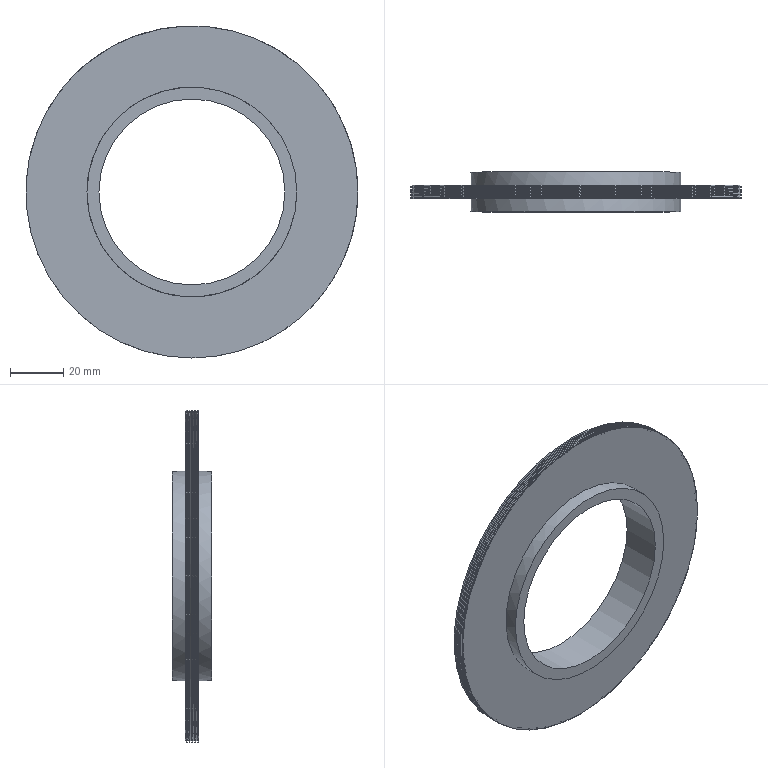Part | NX | features DATUM_CSYS 4, SKETCH 3, EXTRUDE 2, HOLE PACKAGE 1, SIMPLE HOLE 1, SWP104 1 | 1 solid | 33 faces | box 125 x 15 x 125 mm | volume 52069 mm3 | cone 17 | cylinder 12 | plane 4 | commonest cylinder face diameters 125 x9 79 x2 70 x1
STEP:
#1=CARTESIAN_POINT('',(62.5,-10.,0.));
#2=VERTEX_POINT('',#1);
#3=CARTESIAN_POINT('',(0.,-10.,0.));
#4=DIRECTION('',(0.,-1.,0.));
#5=DIRECTION('',(1.,0.,0.));
#6=AXIS2_PLACEMENT_3D('',#3,#4,#5);
#7=CIRCLE('',#6,62.5);
#8=EDGE_CURVE('',#2,#2,#7,.T.);
#9=ORIENTED_EDGE('',*,*,#8,.F.);
#10=EDGE_LOOP('',(#9));
#11=FACE_BOUND('',#10,.T.);
#12=CARTESIAN_POINT('',(0.,-9.824,-62.5));
#13=VERTEX_POINT('',#12);
#14=CARTESIAN_POINT('',(0.,-9.824,0.));
#15=DIRECTION('',(0.,-1.,0.));
#16=DIRECTION('',(0.,0.,-1.));
#17=AXIS2_PLACEMENT_3D('',#14,#15,#16);
#18=CIRCLE('',#17,62.5);
#19=EDGE_CURVE('',#13,#13,#18,.T.);
#20=ORIENTED_EDGE('',*,*,#19,.T.);
#21=EDGE_LOOP('',(#20));
#22=FACE_BOUND('',#21,.T.);
#23=CARTESIAN_POINT('',(0.,-5.,0.));
#24=DIRECTION('',(0.,-1.,0.));
#25=DIRECTION('',(0.,0.,-1.));
#26=AXIS2_PLACEMENT_3D('',#23,#24,#25);
#27=CYLINDRICAL_SURFACE('',#26,62.5);
#28=ADVANCED_FACE('',(#11,#22),#27,.T.);
#29=CARTESIAN_POINT('',(0.,-10.,-39.5));
#30=VERTEX_POINT('',#29);
#31=CARTESIAN_POINT('',(0.,-10.,0.));
#32=DIRECTION('',(0.,-1.,0.));
#33=DIRECTION('',(0.,0.,-1.));
#34=AXIS2_PLACEMENT_3D('',#31,#32,#33);
#35=CIRCLE('',#34,39.5);
#36=EDGE_CURVE('',#30,#30,#35,.T.);
#37=ORIENTED_EDGE('',*,*,#36,.F.);
#38=EDGE_LOOP('',(#37));
#39=FACE_BOUND('',#38,.T.);
#40=ORIENTED_EDGE('',*,*,#8,.T.);
#41=EDGE_LOOP('',(#40));
#42=FACE_BOUND('',#41,.T.);
#43=CARTESIAN_POINT('',(0.,-10.,0.));
#44=DIRECTION('',(0.,-1.,0.));
#45=DIRECTION('',(0.,0.,-1.));
#46=AXIS2_PLACEMENT_3D('',#43,#44,#45);
#47=PLANE('',#46);
#48=ADVANCED_FACE('',(#39,#42),#47,.T.);
#49=CARTESIAN_POINT('',(0.,-15.,35.));
#50=VERTEX_POINT('',#49);
#51=CARTESIAN_POINT('',(0.,-15.,0.));
#52=DIRECTION('',(0.,1.,0.));
#53=DIRECTION('',(0.,0.,1.));
#54=AXIS2_PLACEMENT_3D('',#51,#52,#53);
#55=CIRCLE('',#54,35.);
#56=EDGE_CURVE('',#50,#50,#55,.T.);
#57=ORIENTED_EDGE('',*,*,#56,.T.);
#58=EDGE_LOOP('',(#57));
#59=FACE_BOUND('',#58,.T.);
#60=CARTESIAN_POINT('',(39.5,-15.,0.));
#61=VERTEX_POINT('',#60);
#62=CARTESIAN_POINT('',(0.,-15.,0.));
#63=DIRECTION('',(0.,-1.,0.));
#64=DIRECTION('',(1.,0.,0.));
#65=AXIS2_PLACEMENT_3D('',#62,#63,#64);
#66=CIRCLE('',#65,39.5);
#67=EDGE_CURVE('',#61,#61,#66,.T.);
#68=ORIENTED_EDGE('',*,*,#67,.T.);
#69=EDGE_LOOP('',(#68));
#70=FACE_BOUND('',#69,.T.);
#71=CARTESIAN_POINT('',(0.,-15.,0.));
#72=DIRECTION('',(0.,-1.,0.));
#73=DIRECTION('',(0.,0.,-1.));
#74=AXIS2_PLACEMENT_3D('',#71,#72,#73);
#75=PLANE('',#74);
#76=ADVANCED_FACE('',(#59,#70),#75,.T.);
#77=ORIENTED_EDGE('',*,*,#36,.T.);
#78=EDGE_LOOP('',(#77));
#79=FACE_BOUND('',#78,.T.);
#80=ORIENTED_EDGE('',*,*,#67,.F.);
#81=EDGE_LOOP('',(#80));
#82=FACE_BOUND('',#81,.T.);
#83=CARTESIAN_POINT('',(0.,-15.,0.));
#84=DIRECTION('',(0.,1.,0.));
#85=DIRECTION('',(0.,0.,1.));
#86=AXIS2_PLACEMENT_3D('',#83,#84,#85);
#87=CYLINDRICAL_SURFACE('',#86,39.5);
#88=ADVANCED_FACE('',(#79,#82),#87,.T.);
#89=ORIENTED_EDGE('',*,*,#19,.F.);
#90=EDGE_LOOP('',(#89));
#91=FACE_BOUND('',#90,.T.);
#92=CARTESIAN_POINT('',(0.,-9.628,-61.881));
#93=VERTEX_POINT('',#92);
#94=CARTESIAN_POINT('',(0.,-9.628,0.));
#95=DIRECTION('',(0.,-1.,0.));
#96=DIRECTION('',(0.,0.,-1.));
#97=AXIS2_PLACEMENT_3D('',#94,#95,#96);
#98=CIRCLE('',#97,61.881);
#99=EDGE_CURVE('',#93,#93,#98,.F.);
#100=ORIENTED_EDGE('',*,*,#99,.F.);
#101=EDGE_LOOP('',(#100));
#102=FACE_BOUND('',#101,.T.);
#103=CARTESIAN_POINT('',(0.,-9.825,0.));
#104=DIRECTION('',(0.,-1.,0.));
#105=DIRECTION('',(0.,0.,-1.));
#106=AXIS2_PLACEMENT_3D('',#103,#104,#105);
#107=CONICAL_SURFACE('',#106,62.505,1.264);
#108=ADVANCED_FACE('',(#91,#102),#107,.T.);
#109=CARTESIAN_POINT('',(0.,-9.45,62.5));
#110=VERTEX_POINT('',#109);
#111=CARTESIAN_POINT('',(0.,-9.45,0.));
#112=DIRECTION('',(0.,1.,0.));
#113=DIRECTION('',(0.,0.,1.));
#114=AXIS2_PLACEMENT_3D('',#111,#112,#113);
#115=CIRCLE('',#114,62.5);
#116=EDGE_CURVE('',#110,#110,#115,.T.);
#117=ORIENTED_EDGE('',*,*,#116,.F.);
#118=EDGE_LOOP('',(#117));
#119=FACE_BOUND('',#118,.T.);
#120=ORIENTED_EDGE('',*,*,#99,.T.);
#121=EDGE_LOOP('',(#120));
#122=FACE_BOUND('',#121,.T.);
#123=CARTESIAN_POINT('',(0.,-9.628,0.));
#124=DIRECTION('',(0.,1.,0.));
#125=DIRECTION('',(0.,0.,1.));
#126=AXIS2_PLACEMENT_3D('',#123,#124,#125);
#127=CONICAL_SURFACE('',#126,61.881,1.292);
#128=ADVANCED_FACE('',(#119,#122),#127,.T.);
#129=CARTESIAN_POINT('',(0.,-9.445,-62.5));
#130=VERTEX_POINT('',#129);
#131=CARTESIAN_POINT('',(0.,-9.445,0.));
#132=DIRECTION('',(0.,-1.,0.));
#133=DIRECTION('',(0.,0.,-1.));
#134=AXIS2_PLACEMENT_3D('',#131,#132,#133);
#135=CIRCLE('',#134,62.5);
#136=EDGE_CURVE('',#130,#130,#135,.T.);
#137=ORIENTED_EDGE('',*,*,#136,.T.);
#138=EDGE_LOOP('',(#137));
#139=FACE_BOUND('',#138,.T.);
#140=ORIENTED_EDGE('',*,*,#116,.T.);
#141=EDGE_LOOP('',(#140));
#142=FACE_BOUND('',#141,.T.);
#143=CARTESIAN_POINT('',(0.,-5.,0.));
#144=DIRECTION('',(0.,-1.,0.));
#145=DIRECTION('',(0.,0.,-1.));
#146=AXIS2_PLACEMENT_3D('',#143,#144,#145);
#147=CYLINDRICAL_SURFACE('',#146,62.5);
#148=ADVANCED_FACE('',(#139,#142),#147,.T.);
#149=CARTESIAN_POINT('',(0.,-8.872,62.5));
#150=VERTEX_POINT('',#149);
#151=CARTESIAN_POINT('',(0.,-8.872,0.));
#152=DIRECTION('',(0.,1.,0.));
#153=DIRECTION('',(0.,0.,1.));
#154=AXIS2_PLACEMENT_3D('',#151,#152,#153);
#155=CIRCLE('',#154,62.5);
#156=EDGE_CURVE('',#150,#150,#155,.T.);
#157=ORIENTED_EDGE('',*,*,#156,.F.);
#158=EDGE_LOOP('',(#157));
#159=FACE_BOUND('',#158,.T.);
#160=CARTESIAN_POINT('',(0.,-9.049,-61.881));
#161=VERTEX_POINT('',#160);
#162=CARTESIAN_POINT('',(0.,-9.049,0.));
#163=DIRECTION('',(0.,-1.,0.));
#164=DIRECTION('',(0.,0.,-1.));
#165=AXIS2_PLACEMENT_3D('',#162,#163,#164);
#166=CIRCLE('',#165,61.881);
#167=EDGE_CURVE('',#161,#161,#166,.F.);
#168=ORIENTED_EDGE('',*,*,#167,.T.);
#169=EDGE_LOOP('',(#168));
#170=FACE_BOUND('',#169,.T.);
#171=CARTESIAN_POINT('',(0.,-9.049,0.));
#172=DIRECTION('',(0.,1.,0.));
#173=DIRECTION('',(0.,0.,1.));
#174=AXIS2_PLACEMENT_3D('',#171,#172,#173);
#175=CONICAL_SURFACE('',#174,61.881,1.292);
#176=ADVANCED_FACE('',(#159,#170),#175,.T.);
#177=ORIENTED_EDGE('',*,*,#136,.F.);
#178=EDGE_LOOP('',(#177));
#179=FACE_BOUND('',#178,.T.);
#180=ORIENTED_EDGE('',*,*,#167,.F.);
#181=EDGE_LOOP('',(#180));
#182=FACE_BOUND('',#181,.T.);
#183=CARTESIAN_POINT('',(0.,-9.448,0.));
#184=DIRECTION('',(0.,-1.,0.));
#185=DIRECTION('',(0.,0.,-1.));
#186=AXIS2_PLACEMENT_3D('',#183,#184,#185);
#187=CONICAL_SURFACE('',#186,62.505,1.002);
#188=ADVANCED_FACE('',(#179,#182),#187,.T.);
#189=CARTESIAN_POINT('',(0.,-8.867,-62.5));
#190=VERTEX_POINT('',#189);
#191=CARTESIAN_POINT('',(0.,-8.867,0.));
#192=DIRECTION('',(0.,-1.,0.));
#193=DIRECTION('',(0.,0.,-1.));
#194=AXIS2_PLACEMENT_3D('',#191,#192,#193);
#195=CIRCLE('',#194,62.5);
#196=EDGE_CURVE('',#190,#190,#195,.T.);
#197=ORIENTED_EDGE('',*,*,#196,.T.);
#198=EDGE_LOOP('',(#197));
#199=FACE_BOUND('',#198,.T.);
#200=ORIENTED_EDGE('',*,*,#156,.T.);
#201=EDGE_LOOP('',(#200));
#202=FACE_BOUND('',#201,.T.);
#203=CARTESIAN_POINT('',(0.,-5.,0.));
#204=DIRECTION('',(0.,-1.,0.));
#205=DIRECTION('',(0.,0.,-1.));
#206=AXIS2_PLACEMENT_3D('',#203,#204,#205);
#207=CYLINDRICAL_SURFACE('',#206,62.5);
#208=ADVANCED_FACE('',(#199,#202),#207,.T.);
#209=CARTESIAN_POINT('',(0.,-8.293,62.5));
#210=VERTEX_POINT('',#209);
#211=CARTESIAN_POINT('',(0.,-8.293,0.));
#212=DIRECTION('',(0.,1.,0.));
#213=DIRECTION('',(0.,0.,1.));
#214=AXIS2_PLACEMENT_3D('',#211,#212,#213);
#215=CIRCLE('',#214,62.5);
#216=EDGE_CURVE('',#210,#210,#215,.T.);
#217=ORIENTED_EDGE('',*,*,#216,.F.);
#218=EDGE_LOOP('',(#217));
#219=FACE_BOUND('',#218,.T.);
#220=CARTESIAN_POINT('',(0.,-8.471,-61.881));
#221=VERTEX_POINT('',#220);
#222=CARTESIAN_POINT('',(0.,-8.471,0.));
#223=DIRECTION('',(0.,-1.,0.));
#224=DIRECTION('',(0.,0.,-1.));
#225=AXIS2_PLACEMENT_3D('',#222,#223,#224);
#226=CIRCLE('',#225,61.881);
#227=EDGE_CURVE('',#221,#221,#226,.F.);
#228=ORIENTED_EDGE('',*,*,#227,.T.);
#229=EDGE_LOOP('',(#228));
#230=FACE_BOUND('',#229,.T.);
#231=CARTESIAN_POINT('',(0.,-8.471,0.));
#232=DIRECTION('',(0.,1.,0.));
#233=DIRECTION('',(0.,0.,1.));
#234=AXIS2_PLACEMENT_3D('',#231,#232,#233);
#235=CONICAL_SURFACE('',#234,61.881,1.292);
#236=ADVANCED_FACE('',(#219,#230),#235,.T.);
#237=ORIENTED_EDGE('',*,*,#196,.F.);
#238=EDGE_LOOP('',(#237));
#239=FACE_BOUND('',#238,.T.);
#240=ORIENTED_EDGE('',*,*,#227,.F.);
#241=EDGE_LOOP('',(#240));
#242=FACE_BOUND('',#241,.T.);
#243=CARTESIAN_POINT('',(0.,-8.87,0.));
#244=DIRECTION('',(0.,-1.,0.));
#245=DIRECTION('',(0.,0.,-1.));
#246=AXIS2_PLACEMENT_3D('',#243,#244,#245);
#247=CONICAL_SURFACE('',#246,62.505,1.002);
#248=ADVANCED_FACE('',(#239,#242),#247,.T.);
#249=CARTESIAN_POINT('',(0.,-8.288,-62.5));
#250=VERTEX_POINT('',#249);
#251=CARTESIAN_POINT('',(0.,-8.288,0.));
#252=DIRECTION('',(0.,-1.,0.));
#253=DIRECTION('',(0.,0.,-1.));
#254=AXIS2_PLACEMENT_3D('',#251,#252,#253);
#255=CIRCLE('',#254,62.5);
#256=EDGE_CURVE('',#250,#250,#255,.T.);
#257=ORIENTED_EDGE('',*,*,#256,.T.);
#258=EDGE_LOOP('',(#257));
#259=FACE_BOUND('',#258,.T.);
#260=ORIENTED_EDGE('',*,*,#216,.T.);
#261=EDGE_LOOP('',(#260));
#262=FACE_BOUND('',#261,.T.);
#263=CARTESIAN_POINT('',(0.,-5.,0.));
#264=DIRECTION('',(0.,-1.,0.));
#265=DIRECTION('',(0.,0.,-1.));
#266=AXIS2_PLACEMENT_3D('',#263,#264,#265);
#267=CYLINDRICAL_SURFACE('',#266,62.5);
#268=ADVANCED_FACE('',(#259,#262),#267,.T.);
#269=CARTESIAN_POINT('',(0.,-7.715,62.5));
#270=VERTEX_POINT('',#269);
#271=CARTESIAN_POINT('',(0.,-7.715,0.));
#272=DIRECTION('',(0.,1.,0.));
#273=DIRECTION('',(0.,0.,1.));
#274=AXIS2_PLACEMENT_3D('',#271,#272,#273);
#275=CIRCLE('',#274,62.5);
#276=EDGE_CURVE('',#270,#270,#275,.T.);
#277=ORIENTED_EDGE('',*,*,#276,.F.);
#278=EDGE_LOOP('',(#277));
#279=FACE_BOUND('',#278,.T.);
#280=CARTESIAN_POINT('',(0.,-7.892,-61.881));
#281=VERTEX_POINT('',#280);
#282=CARTESIAN_POINT('',(0.,-7.892,0.));
#283=DIRECTION('',(0.,-1.,0.));
#284=DIRECTION('',(0.,0.,-1.));
#285=AXIS2_PLACEMENT_3D('',#282,#283,#284);
#286=CIRCLE('',#285,61.881);
#287=EDGE_CURVE('',#281,#281,#286,.F.);
#288=ORIENTED_EDGE('',*,*,#287,.T.);
#289=EDGE_LOOP('',(#288));
#290=FACE_BOUND('',#289,.T.);
#291=CARTESIAN_POINT('',(0.,-7.892,0.));
#292=DIRECTION('',(0.,1.,0.));
#293=DIRECTION('',(0.,0.,1.));
#294=AXIS2_PLACEMENT_3D('',#291,#292,#293);
#295=CONICAL_SURFACE('',#294,61.881,1.292);
#296=ADVANCED_FACE('',(#279,#290),#295,.T.);
#297=ORIENTED_EDGE('',*,*,#256,.F.);
#298=EDGE_LOOP('',(#297));
#299=FACE_BOUND('',#298,.T.);
#300=ORIENTED_EDGE('',*,*,#287,.F.);
#301=EDGE_LOOP('',(#300));
#302=FACE_BOUND('',#301,.T.);
#303=CARTESIAN_POINT('',(0.,-8.292,0.));
#304=DIRECTION('',(0.,-1.,0.));
#305=DIRECTION('',(0.,0.,-1.));
#306=AXIS2_PLACEMENT_3D('',#303,#304,#305);
#307=CONICAL_SURFACE('',#306,62.505,1.002);
#308=ADVANCED_FACE('',(#299,#302),#307,.T.);
#309=CARTESIAN_POINT('',(0.,-7.71,-62.5));
#310=VERTEX_POINT('',#309);
#311=CARTESIAN_POINT('',(0.,-7.71,0.));
#312=DIRECTION('',(0.,-1.,0.));
#313=DIRECTION('',(0.,0.,-1.));
#314=AXIS2_PLACEMENT_3D('',#311,#312,#313);
#315=CIRCLE('',#314,62.5);
#316=EDGE_CURVE('',#310,#310,#315,.T.);
#317=ORIENTED_EDGE('',*,*,#316,.T.);
#318=EDGE_LOOP('',(#317));
#319=FACE_BOUND('',#318,.T.);
#320=ORIENTED_EDGE('',*,*,#276,.T.);
#321=EDGE_LOOP('',(#320));
#322=FACE_BOUND('',#321,.T.);
#323=CARTESIAN_POINT('',(0.,-5.,0.));
#324=DIRECTION('',(0.,-1.,0.));
#325=DIRECTION('',(0.,0.,-1.));
#326=AXIS2_PLACEMENT_3D('',#323,#324,#325);
#327=CYLINDRICAL_SURFACE('',#326,62.5);
#328=ADVANCED_FACE('',(#319,#322),#327,.T.);
#329=CARTESIAN_POINT('',(0.,-7.136,62.5));
#330=VERTEX_POINT('',#329);
#331=CARTESIAN_POINT('',(0.,-7.136,0.));
#332=DIRECTION('',(0.,1.,0.));
#333=DIRECTION('',(0.,0.,1.));
#334=AXIS2_PLACEMENT_3D('',#331,#332,#333);
#335=CIRCLE('',#334,62.5);
#336=EDGE_CURVE('',#330,#330,#335,.T.);
#337=ORIENTED_EDGE('',*,*,#336,.F.);
#338=EDGE_LOOP('',(#337));
#339=FACE_BOUND('',#338,.T.);
#340=CARTESIAN_POINT('',(0.,-7.314,-61.881));
#341=VERTEX_POINT('',#340);
#342=CARTESIAN_POINT('',(0.,-7.314,0.));
#343=DIRECTION('',(0.,-1.,0.));
#344=DIRECTION('',(0.,0.,-1.));
#345=AXIS2_PLACEMENT_3D('',#342,#343,#344);
#346=CIRCLE('',#345,61.881);
#347=EDGE_CURVE('',#341,#341,#346,.F.);
#348=ORIENTED_EDGE('',*,*,#347,.T.);
#349=EDGE_LOOP('',(#348));
#350=FACE_BOUND('',#349,.T.);
#351=CARTESIAN_POINT('',(0.,-7.314,0.));
#352=DIRECTION('',(0.,1.,0.));
#353=DIRECTION('',(0.,0.,1.));
#354=AXIS2_PLACEMENT_3D('',#351,#352,#353);
#355=CONICAL_SURFACE('',#354,61.881,1.292);
#356=ADVANCED_FACE('',(#339,#350),#355,.T.);
#357=ORIENTED_EDGE('',*,*,#316,.F.);
#358=EDGE_LOOP('',(#357));
#359=FACE_BOUND('',#358,.T.);
#360=ORIENTED_EDGE('',*,*,#347,.F.);
#361=EDGE_LOOP('',(#360));
#362=FACE_BOUND('',#361,.T.);
#363=CARTESIAN_POINT('',(0.,-7.713,0.));
#364=DIRECTION('',(0.,-1.,0.));
#365=DIRECTION('',(0.,0.,-1.));
#366=AXIS2_PLACEMENT_3D('',#363,#364,#365);
#367=CONICAL_SURFACE('',#366,62.505,1.002);
#368=ADVANCED_FACE('',(#359,#362),#367,.T.);
#369=CARTESIAN_POINT('',(0.,-7.131,-62.5));
#370=VERTEX_POINT('',#369);
#371=CARTESIAN_POINT('',(0.,-7.131,0.));
#372=DIRECTION('',(0.,-1.,0.));
#373=DIRECTION('',(0.,0.,-1.));
#374=AXIS2_PLACEMENT_3D('',#371,#372,#373);
#375=CIRCLE('',#374,62.5);
#376=EDGE_CURVE('',#370,#370,#375,.T.);
#377=ORIENTED_EDGE('',*,*,#376,.T.);
#378=EDGE_LOOP('',(#377));
#379=FACE_BOUND('',#378,.T.);
#380=ORIENTED_EDGE('',*,*,#336,.T.);
#381=EDGE_LOOP('',(#380));
#382=FACE_BOUND('',#381,.T.);
#383=CARTESIAN_POINT('',(0.,-5.,0.));
#384=DIRECTION('',(0.,-1.,0.));
#385=DIRECTION('',(0.,0.,-1.));
#386=AXIS2_PLACEMENT_3D('',#383,#384,#385);
#387=CYLINDRICAL_SURFACE('',#386,62.5);
#388=ADVANCED_FACE('',(#379,#382),#387,.T.);
#389=CARTESIAN_POINT('',(0.,-6.558,62.5));
#390=VERTEX_POINT('',#389);
#391=CARTESIAN_POINT('',(0.,-6.558,0.));
#392=DIRECTION('',(0.,1.,0.));
#393=DIRECTION('',(0.,0.,1.));
#394=AXIS2_PLACEMENT_3D('',#391,#392,#393);
#395=CIRCLE('',#394,62.5);
#396=EDGE_CURVE('',#390,#390,#395,.T.);
#397=ORIENTED_EDGE('',*,*,#396,.F.);
#398=EDGE_LOOP('',(#397));
#399=FACE_BOUND('',#398,.T.);
#400=CARTESIAN_POINT('',(0.,-6.735,-61.881));
#401=VERTEX_POINT('',#400);
#402=CARTESIAN_POINT('',(0.,-6.735,0.));
#403=DIRECTION('',(0.,-1.,0.));
#404=DIRECTION('',(0.,0.,-1.));
#405=AXIS2_PLACEMENT_3D('',#402,#403,#404);
#406=CIRCLE('',#405,61.881);
#407=EDGE_CURVE('',#401,#401,#406,.F.);
#408=ORIENTED_EDGE('',*,*,#407,.T.);
#409=EDGE_LOOP('',(#408));
#410=FACE_BOUND('',#409,.T.);
#411=CARTESIAN_POINT('',(0.,-6.735,0.));
#412=DIRECTION('',(0.,1.,0.));
#413=DIRECTION('',(0.,0.,1.));
#414=AXIS2_PLACEMENT_3D('',#411,#412,#413);
#415=CONICAL_SURFACE('',#414,61.881,1.292);
#416=ADVANCED_FACE('',(#399,#410),#415,.T.);
#417=ORIENTED_EDGE('',*,*,#376,.F.);
#418=EDGE_LOOP('',(#417));
#419=FACE_BOUND('',#418,.T.);
#420=ORIENTED_EDGE('',*,*,#407,.F.);
#421=EDGE_LOOP('',(#420));
#422=FACE_BOUND('',#421,.T.);
#423=CARTESIAN_POINT('',(0.,-7.135,0.));
#424=DIRECTION('',(0.,-1.,0.));
#425=DIRECTION('',(0.,0.,-1.));
#426=AXIS2_PLACEMENT_3D('',#423,#424,#425);
#427=CONICAL_SURFACE('',#426,62.505,1.002);
#428=ADVANCED_FACE('',(#419,#422),#427,.T.);
#429=CARTESIAN_POINT('',(0.,-6.553,-62.5));
#430=VERTEX_POINT('',#429);
#431=CARTESIAN_POINT('',(0.,-6.553,0.));
#432=DIRECTION('',(0.,-1.,0.));
#433=DIRECTION('',(0.,0.,-1.));
#434=AXIS2_PLACEMENT_3D('',#431,#432,#433);
#435=CIRCLE('',#434,62.5);
#436=EDGE_CURVE('',#430,#430,#435,.T.);
#437=ORIENTED_EDGE('',*,*,#436,.T.);
#438=EDGE_LOOP('',(#437));
#439=FACE_BOUND('',#438,.T.);
#440=ORIENTED_EDGE('',*,*,#396,.T.);
#441=EDGE_LOOP('',(#440));
#442=FACE_BOUND('',#441,.T.);
#443=CARTESIAN_POINT('',(0.,-5.,0.));
#444=DIRECTION('',(0.,-1.,0.));
#445=DIRECTION('',(0.,0.,-1.));
#446=AXIS2_PLACEMENT_3D('',#443,#444,#445);
#447=CYLINDRICAL_SURFACE('',#446,62.5);
#448=ADVANCED_FACE('',(#439,#442),#447,.T.);
#449=CARTESIAN_POINT('',(0.,-5.979,62.5));
#450=VERTEX_POINT('',#449);
#451=CARTESIAN_POINT('',(0.,-5.979,0.));
#452=DIRECTION('',(0.,1.,0.));
#453=DIRECTION('',(0.,0.,1.));
#454=AXIS2_PLACEMENT_3D('',#451,#452,#453);
#455=CIRCLE('',#454,62.5);
#456=EDGE_CURVE('',#450,#450,#455,.T.);
#457=ORIENTED_EDGE('',*,*,#456,.F.);
#458=EDGE_LOOP('',(#457));
#459=FACE_BOUND('',#458,.T.);
#460=CARTESIAN_POINT('',(0.,-6.157,-61.881));
#461=VERTEX_POINT('',#460);
#462=CARTESIAN_POINT('',(0.,-6.157,0.));
#463=DIRECTION('',(0.,-1.,0.));
#464=DIRECTION('',(0.,0.,-1.));
#465=AXIS2_PLACEMENT_3D('',#462,#463,#464);
#466=CIRCLE('',#465,61.881);
#467=EDGE_CURVE('',#461,#461,#466,.F.);
#468=ORIENTED_EDGE('',*,*,#467,.T.);
#469=EDGE_LOOP('',(#468));
#470=FACE_BOUND('',#469,.T.);
#471=CARTESIAN_POINT('',(0.,-6.157,0.));
#472=DIRECTION('',(0.,1.,0.));
#473=DIRECTION('',(0.,0.,1.));
#474=AXIS2_PLACEMENT_3D('',#471,#472,#473);
#475=CONICAL_SURFACE('',#474,61.881,1.292);
#476=ADVANCED_FACE('',(#459,#470),#475,.T.);
#477=ORIENTED_EDGE('',*,*,#436,.F.);
#478=EDGE_LOOP('',(#477));
#479=FACE_BOUND('',#478,.T.);
#480=ORIENTED_EDGE('',*,*,#467,.F.);
#481=EDGE_LOOP('',(#480));
#482=FACE_BOUND('',#481,.T.);
#483=CARTESIAN_POINT('',(0.,-6.556,0.));
#484=DIRECTION('',(0.,-1.,0.));
#485=DIRECTION('',(0.,0.,-1.));
#486=AXIS2_PLACEMENT_3D('',#483,#484,#485);
#487=CONICAL_SURFACE('',#486,62.505,1.002);
#488=ADVANCED_FACE('',(#479,#482),#487,.T.);
#489=CARTESIAN_POINT('',(0.,-5.974,-62.5));
#490=VERTEX_POINT('',#489);
#491=CARTESIAN_POINT('',(0.,-5.974,0.));
#492=DIRECTION('',(0.,-1.,0.));
#493=DIRECTION('',(0.,0.,-1.));
#494=AXIS2_PLACEMENT_3D('',#491,#492,#493);
#495=CIRCLE('',#494,62.5);
#496=EDGE_CURVE('',#490,#490,#495,.T.);
#497=ORIENTED_EDGE('',*,*,#496,.T.);
#498=EDGE_LOOP('',(#497));
#499=FACE_BOUND('',#498,.T.);
#500=ORIENTED_EDGE('',*,*,#456,.T.);
#501=EDGE_LOOP('',(#500));
#502=FACE_BOUND('',#501,.T.);
#503=CARTESIAN_POINT('',(0.,-5.,0.));
#504=DIRECTION('',(0.,-1.,0.));
#505=DIRECTION('',(0.,0.,-1.));
#506=AXIS2_PLACEMENT_3D('',#503,#504,#505);
#507=CYLINDRICAL_SURFACE('',#506,62.5);
#508=ADVANCED_FACE('',(#499,#502),#507,.T.);
#509=CARTESIAN_POINT('',(0.,-5.401,62.5));
#510=VERTEX_POINT('',#509);
#511=CARTESIAN_POINT('',(0.,-5.401,0.));
#512=DIRECTION('',(0.,1.,0.));
#513=DIRECTION('',(0.,0.,1.));
#514=AXIS2_PLACEMENT_3D('',#511,#512,#513);
#515=CIRCLE('',#514,62.5);
#516=EDGE_CURVE('',#510,#510,#515,.T.);
#517=ORIENTED_EDGE('',*,*,#516,.F.);
#518=EDGE_LOOP('',(#517));
#519=FACE_BOUND('',#518,.T.);
#520=CARTESIAN_POINT('',(0.,-5.578,-61.881));
#521=VERTEX_POINT('',#520);
#522=CARTESIAN_POINT('',(0.,-5.578,0.));
#523=DIRECTION('',(0.,-1.,0.));
#524=DIRECTION('',(0.,0.,-1.));
#525=AXIS2_PLACEMENT_3D('',#522,#523,#524);
#526=CIRCLE('',#525,61.881);
#527=EDGE_CURVE('',#521,#521,#526,.F.);
#528=ORIENTED_EDGE('',*,*,#527,.T.);
#529=EDGE_LOOP('',(#528));
#530=FACE_BOUND('',#529,.T.);
#531=CARTESIAN_POINT('',(0.,-5.578,0.));
#532=DIRECTION('',(0.,1.,0.));
#533=DIRECTION('',(0.,0.,1.));
#534=AXIS2_PLACEMENT_3D('',#531,#532,#533);
#535=CONICAL_SURFACE('',#534,61.881,1.292);
#536=ADVANCED_FACE('',(#519,#530),#535,.T.);
#537=ORIENTED_EDGE('',*,*,#496,.F.);
#538=EDGE_LOOP('',(#537));
#539=FACE_BOUND('',#538,.T.);
#540=ORIENTED_EDGE('',*,*,#527,.F.);
#541=EDGE_LOOP('',(#540));
#542=FACE_BOUND('',#541,.T.);
#543=CARTESIAN_POINT('',(0.,-5.978,0.));
#544=DIRECTION('',(0.,-1.,0.));
#545=DIRECTION('',(0.,0.,-1.));
#546=AXIS2_PLACEMENT_3D('',#543,#544,#545);
#547=CONICAL_SURFACE('',#546,62.505,1.002);
#548=ADVANCED_FACE('',(#539,#542),#547,.T.);
#549=CARTESIAN_POINT('',(0.,-5.396,-62.5));
#550=VERTEX_POINT('',#549);
#551=CARTESIAN_POINT('',(0.,-5.396,0.));
#552=DIRECTION('',(0.,-1.,0.));
#553=DIRECTION('',(0.,0.,-1.));
#554=AXIS2_PLACEMENT_3D('',#551,#552,#553);
#555=CIRCLE('',#554,62.5);
#556=EDGE_CURVE('',#550,#550,#555,.T.);
#557=ORIENTED_EDGE('',*,*,#556,.T.);
#558=EDGE_LOOP('',(#557));
#559=FACE_BOUND('',#558,.T.);
#560=ORIENTED_EDGE('',*,*,#516,.T.);
#561=EDGE_LOOP('',(#560));
#562=FACE_BOUND('',#561,.T.);
#563=CARTESIAN_POINT('',(0.,-5.,0.));
#564=DIRECTION('',(0.,-1.,0.));
#565=DIRECTION('',(0.,0.,-1.));
#566=AXIS2_PLACEMENT_3D('',#563,#564,#565);
#567=CYLINDRICAL_SURFACE('',#566,62.5);
#568=ADVANCED_FACE('',(#559,#562),#567,.T.);
#569=ORIENTED_EDGE('',*,*,#556,.F.);
#570=EDGE_LOOP('',(#569));
#571=FACE_BOUND('',#570,.T.);
#572=CARTESIAN_POINT('',(0.,-5.,-61.881));
#573=VERTEX_POINT('',#572);
#574=CARTESIAN_POINT('',(0.,-5.,0.));
#575=DIRECTION('',(0.,-1.,0.));
#576=DIRECTION('',(0.,0.,-1.));
#577=AXIS2_PLACEMENT_3D('',#574,#575,#576);
#578=CIRCLE('',#577,61.881);
#579=EDGE_CURVE('',#573,#573,#578,.T.);
#580=ORIENTED_EDGE('',*,*,#579,.T.);
#581=EDGE_LOOP('',(#580));
#582=FACE_BOUND('',#581,.T.);
#583=CARTESIAN_POINT('',(0.,-5.399,0.));
#584=DIRECTION('',(0.,-1.,0.));
#585=DIRECTION('',(0.,0.,-1.));
#586=AXIS2_PLACEMENT_3D('',#583,#584,#585);
#587=CONICAL_SURFACE('',#586,62.505,1.002);
#588=ADVANCED_FACE('',(#571,#582),#587,.T.);
#589=CARTESIAN_POINT('',(0.,0.,-35.));
#590=VERTEX_POINT('',#589);
#591=CARTESIAN_POINT('',(0.,0.,0.));
#592=DIRECTION('',(0.,-1.,0.));
#593=DIRECTION('',(0.,0.,-1.));
#594=AXIS2_PLACEMENT_3D('',#591,#592,#593);
#595=CIRCLE('',#594,35.);
#596=EDGE_CURVE('',#590,#590,#595,.T.);
#597=ORIENTED_EDGE('',*,*,#596,.T.);
#598=EDGE_LOOP('',(#597));
#599=FACE_BOUND('',#598,.T.);
#600=CARTESIAN_POINT('',(39.5,0.,0.));
#601=VERTEX_POINT('',#600);
#602=CARTESIAN_POINT('',(0.,0.,0.));
#603=DIRECTION('',(0.,-1.,0.));
#604=DIRECTION('',(1.,0.,0.));
#605=AXIS2_PLACEMENT_3D('',#602,#603,#604);
#606=CIRCLE('',#605,39.5);
#607=EDGE_CURVE('',#601,#601,#606,.T.);
#608=ORIENTED_EDGE('',*,*,#607,.F.);
#609=EDGE_LOOP('',(#608));
#610=FACE_BOUND('',#609,.T.);
#611=CARTESIAN_POINT('',(0.,0.,0.));
#612=DIRECTION('',(0.,-1.,0.));
#613=DIRECTION('',(0.,0.,-1.));
#614=AXIS2_PLACEMENT_3D('',#611,#612,#613);
#615=PLANE('',#614);
#616=ADVANCED_FACE('',(#599,#610),#615,.F.);
#617=ORIENTED_EDGE('',*,*,#607,.T.);
#618=EDGE_LOOP('',(#617));
#619=FACE_BOUND('',#618,.T.);
#620=CARTESIAN_POINT('',(0.,-5.,-39.5));
#621=VERTEX_POINT('',#620);
#622=CARTESIAN_POINT('',(0.,-5.,0.));
#623=DIRECTION('',(0.,-1.,0.));
#624=DIRECTION('',(0.,0.,-1.));
#625=AXIS2_PLACEMENT_3D('',#622,#623,#624);
#626=CIRCLE('',#625,39.5);
#627=EDGE_CURVE('',#621,#621,#626,.T.);
#628=ORIENTED_EDGE('',*,*,#627,.F.);
#629=EDGE_LOOP('',(#628));
#630=FACE_BOUND('',#629,.T.);
#631=CARTESIAN_POINT('',(0.,-15.,0.));
#632=DIRECTION('',(0.,1.,0.));
#633=DIRECTION('',(0.,0.,1.));
#634=AXIS2_PLACEMENT_3D('',#631,#632,#633);
#635=CYLINDRICAL_SURFACE('',#634,39.5);
#636=ADVANCED_FACE('',(#619,#630),#635,.T.);
#637=ORIENTED_EDGE('',*,*,#627,.T.);
#638=EDGE_LOOP('',(#637));
#639=FACE_BOUND('',#638,.T.);
#640=ORIENTED_EDGE('',*,*,#579,.F.);
#641=EDGE_LOOP('',(#640));
#642=FACE_BOUND('',#641,.T.);
#643=CARTESIAN_POINT('',(0.,-5.,0.));
#644=DIRECTION('',(0.,-1.,0.));
#645=DIRECTION('',(0.,0.,-1.));
#646=AXIS2_PLACEMENT_3D('',#643,#644,#645);
#647=PLANE('',#646);
#648=ADVANCED_FACE('',(#639,#642),#647,.F.);
#649=ORIENTED_EDGE('',*,*,#56,.F.);
#650=EDGE_LOOP('',(#649));
#651=FACE_BOUND('',#650,.T.);
#652=ORIENTED_EDGE('',*,*,#596,.F.);
#653=EDGE_LOOP('',(#652));
#654=FACE_BOUND('',#653,.T.);
#655=CARTESIAN_POINT('',(0.,-15.,0.));
#656=DIRECTION('',(0.,1.,0.));
#657=DIRECTION('',(0.,0.,1.));
#658=AXIS2_PLACEMENT_3D('',#655,#656,#657);
#659=CYLINDRICAL_SURFACE('',#658,35.);
#660=ADVANCED_FACE('',(#651,#654),#659,.F.);
#661=CLOSED_SHELL('',(#28,#48,#76,#88,#108,#128,#148,#176,#188,#208,#236,#248,#268,#296,#308,#328,#356,#368,#388,#416,#428,#448,#476,#488,#508,#536,#548,#568,#588,#616,#636,#648,#660));
#662=MANIFOLD_SOLID_BREP('',#661);
#663=(LENGTH_UNIT()NAMED_UNIT(*)SI_UNIT(.MILLI.,.METRE.));
#664=UNCERTAINTY_MEASURE_WITH_UNIT(LENGTH_MEASURE(0.00001),#663,'','');
#665=(NAMED_UNIT(*)PLANE_ANGLE_UNIT()SI_UNIT($,.RADIAN.));
#666=(NAMED_UNIT(*)SI_UNIT($,.STERADIAN.)SOLID_ANGLE_UNIT());
#667=(GEOMETRIC_REPRESENTATION_CONTEXT(3)GLOBAL_UNCERTAINTY_ASSIGNED_CONTEXT((#664))GLOBAL_UNIT_ASSIGNED_CONTEXT((#663,#665,#666))REPRESENTATION_CONTEXT('',''));
#668=ADVANCED_BREP_SHAPE_REPRESENTATION('',(#662),#667);